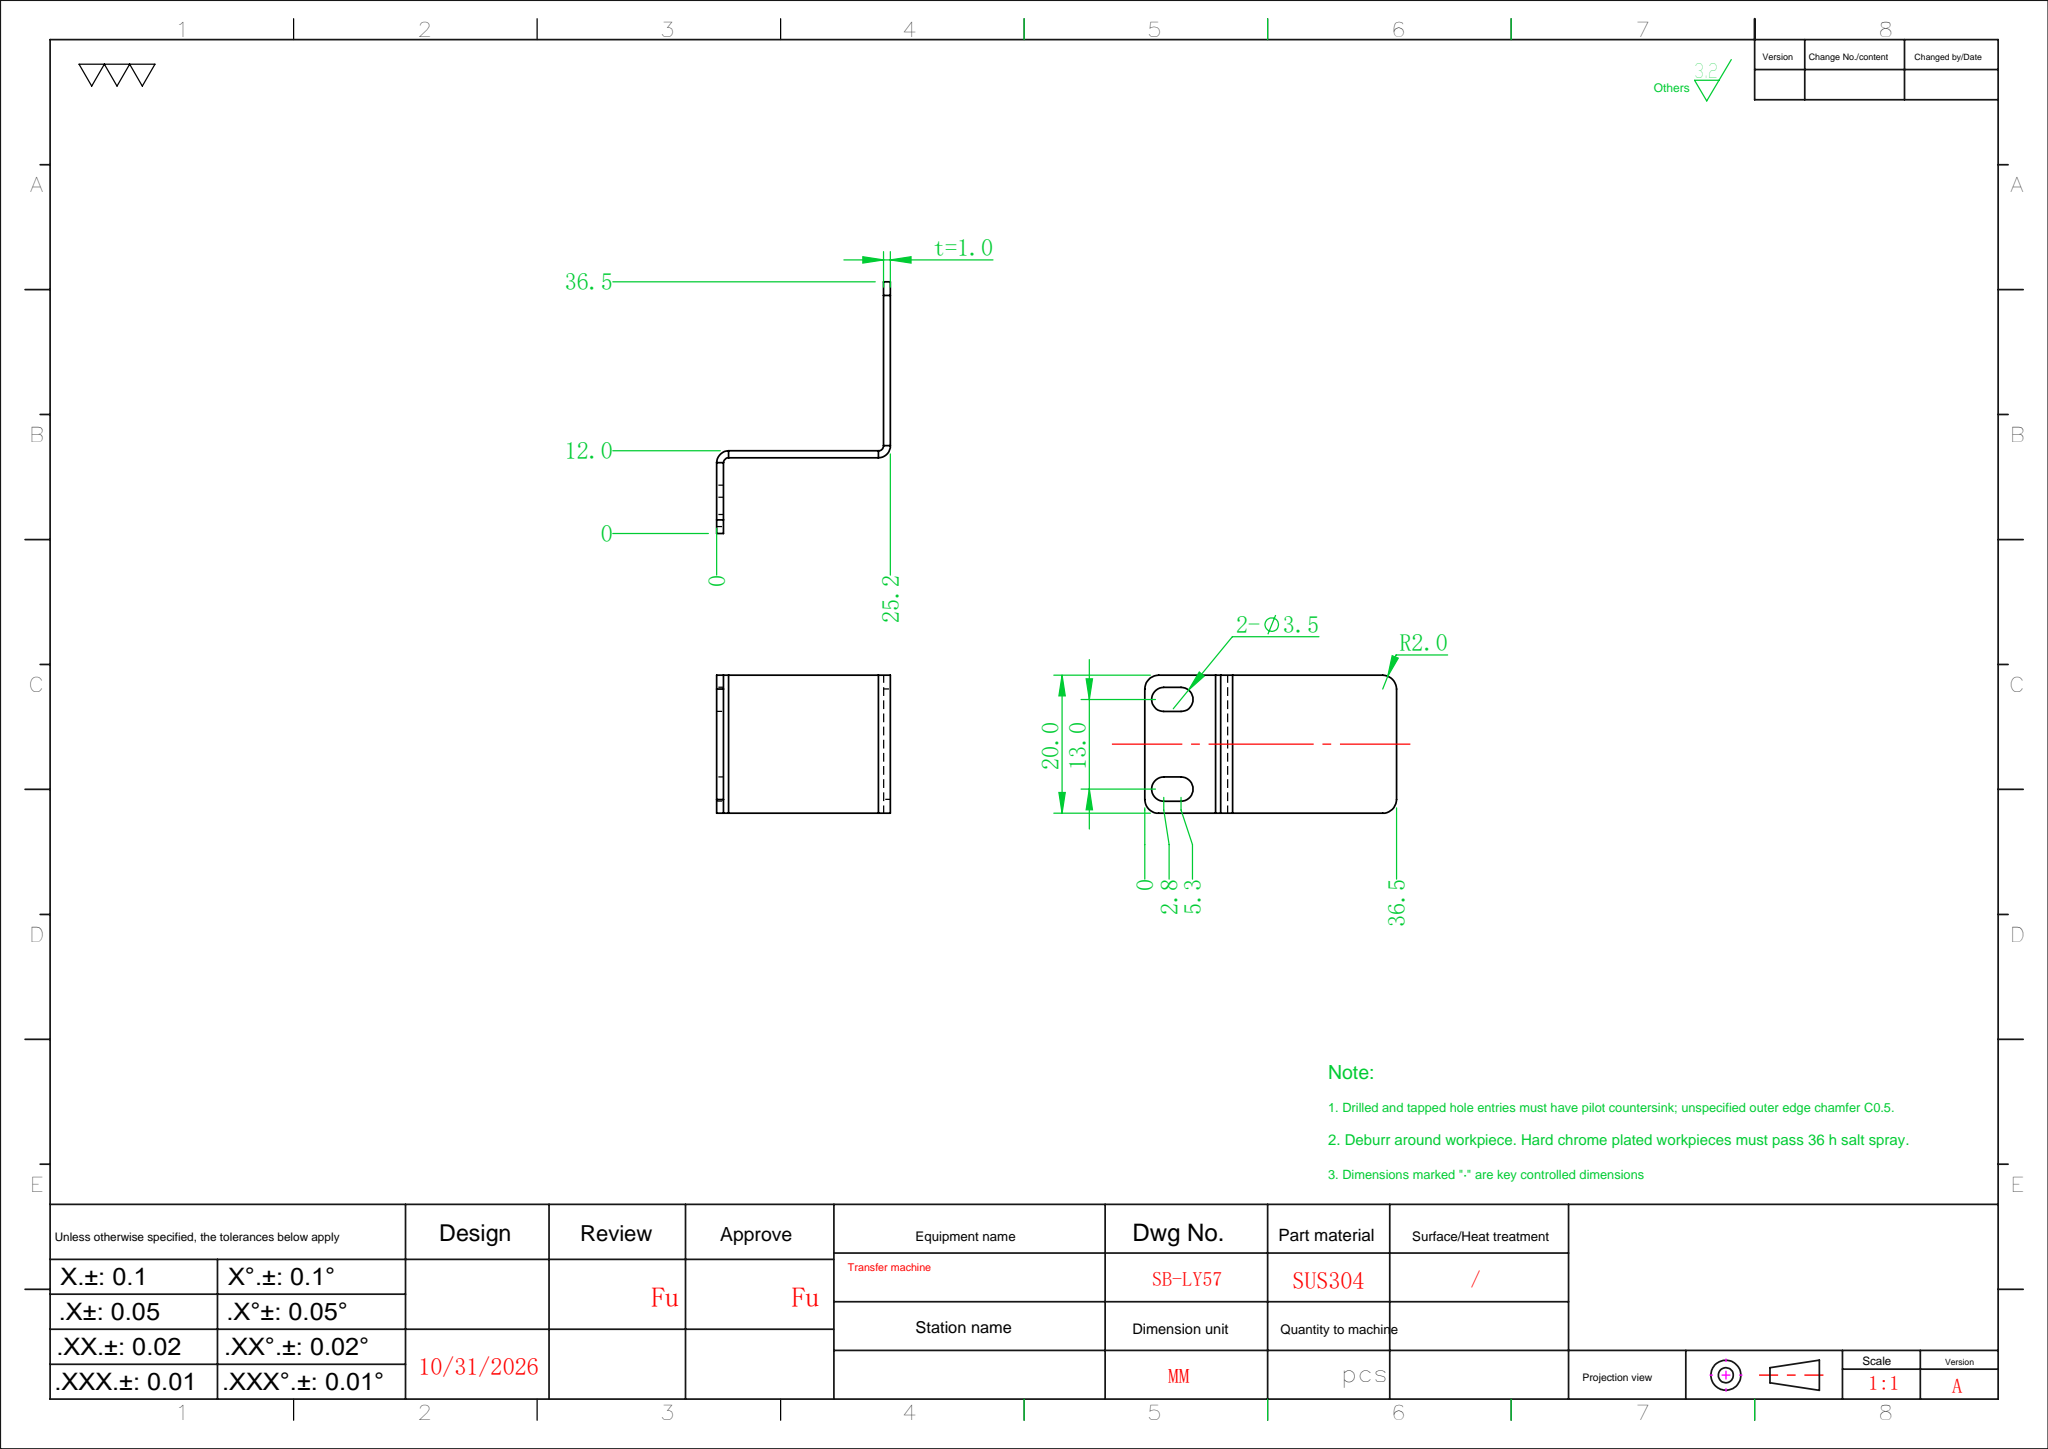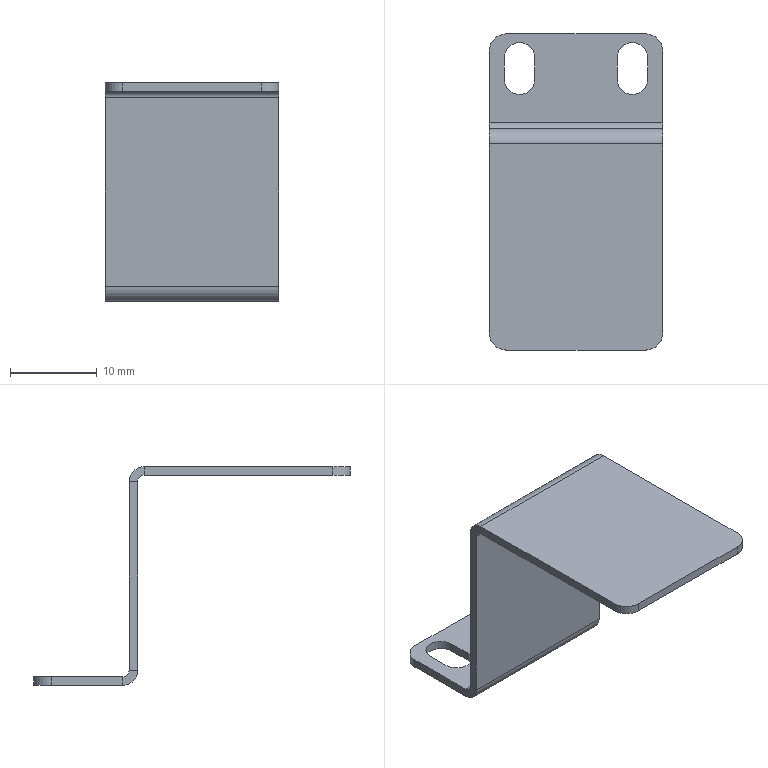Part | SolidWorks | features EdgeFlange 2, Fillet 1, FlatPattern 1, HoleWzd 1, SMBaseFlange 1, SheetMetal 1 | 1 solid | 34 faces | box 20 x 36.5 x 25.2 mm | volume 1153 mm3 | plane 22 | cylinder 12 | commonest cylinder face diameters 3.5 x4 4 x4 1.473 x2 3.473 x2
STEP:
#1=CARTESIAN_POINT('',(-10.,-6.,22.463));
#2=VERTEX_POINT('',#1);
#3=CARTESIAN_POINT('',(-10.,-5.,22.463));
#4=VERTEX_POINT('',#3);
#5=CARTESIAN_POINT('',(-10.,-6.,22.463));
#6=DIRECTION('',(0.,1.,0.));
#7=VECTOR('',#6,1000.);
#8=LINE('',#5,#7);
#9=EDGE_CURVE('',#2,#4,#8,.T.);
#10=ORIENTED_EDGE('',*,*,#9,.T.);
#11=CARTESIAN_POINT('',(-10.,-5.,0.7366));
#12=VERTEX_POINT('',#11);
#13=CARTESIAN_POINT('',(-10.,-5.,0.));
#14=DIRECTION('',(0.,0.,-1.));
#15=VECTOR('',#14,1000.);
#16=LINE('',#13,#15);
#17=EDGE_CURVE('',#4,#12,#16,.T.);
#18=ORIENTED_EDGE('',*,*,#17,.T.);
#19=CARTESIAN_POINT('',(-10.,-6.,0.7366));
#20=VERTEX_POINT('',#19);
#21=CARTESIAN_POINT('',(-10.,-6.,0.7366));
#22=DIRECTION('',(0.,-1.,0.));
#23=VECTOR('',#22,1000.);
#24=LINE('',#21,#23);
#25=EDGE_CURVE('',#12,#20,#24,.T.);
#26=ORIENTED_EDGE('',*,*,#25,.T.);
#27=CARTESIAN_POINT('',(-10.,-6.,0.));
#28=DIRECTION('',(0.,0.,-1.));
#29=VECTOR('',#28,1000.);
#30=LINE('',#27,#29);
#31=EDGE_CURVE('',#2,#20,#30,.T.);
#32=ORIENTED_EDGE('',*,*,#31,.F.);
#33=EDGE_LOOP('',(#10,#18,#26,#32));
#34=FACE_OUTER_BOUND('',#33,.T.);
#35=CARTESIAN_POINT('',(-10.,-6.,0.));
#36=DIRECTION('',(1.,0.,0.));
#37=DIRECTION('',(0.,0.,-1.));
#38=AXIS2_PLACEMENT_3D('',#35,#36,#37);
#39=PLANE('',#38);
#40=ADVANCED_FACE('',(#34),#39,.F.);
#41=CARTESIAN_POINT('',(10.,-6.,22.463));
#42=VERTEX_POINT('',#41);
#43=CARTESIAN_POINT('',(10.,-5.,22.463));
#44=VERTEX_POINT('',#43);
#45=CARTESIAN_POINT('',(10.,-6.,22.463));
#46=DIRECTION('',(0.,1.,0.));
#47=VECTOR('',#46,1000.);
#48=LINE('',#45,#47);
#49=EDGE_CURVE('',#42,#44,#48,.T.);
#50=ORIENTED_EDGE('',*,*,#49,.F.);
#51=CARTESIAN_POINT('',(10.,-6.,0.7366));
#52=VERTEX_POINT('',#51);
#53=CARTESIAN_POINT('',(10.,-6.,0.));
#54=DIRECTION('',(0.,0.,1.));
#55=VECTOR('',#54,1000.);
#56=LINE('',#53,#55);
#57=EDGE_CURVE('',#52,#42,#56,.T.);
#58=ORIENTED_EDGE('',*,*,#57,.F.);
#59=CARTESIAN_POINT('',(10.,-5.,0.7366));
#60=VERTEX_POINT('',#59);
#61=CARTESIAN_POINT('',(10.,-5.,0.7366));
#62=DIRECTION('',(0.,-1.,0.));
#63=VECTOR('',#62,1000.);
#64=LINE('',#61,#63);
#65=EDGE_CURVE('',#60,#52,#64,.T.);
#66=ORIENTED_EDGE('',*,*,#65,.F.);
#67=CARTESIAN_POINT('',(10.,-5.,24.2));
#68=DIRECTION('',(0.,0.,1.));
#69=VECTOR('',#68,1000.);
#70=LINE('',#67,#69);
#71=EDGE_CURVE('',#60,#44,#70,.T.);
#72=ORIENTED_EDGE('',*,*,#71,.T.);
#73=EDGE_LOOP('',(#50,#58,#66,#72));
#74=FACE_OUTER_BOUND('',#73,.T.);
#75=CARTESIAN_POINT('',(10.,-6.,24.2));
#76=DIRECTION('',(-1.,0.,0.));
#77=DIRECTION('',(0.,0.,1.));
#78=AXIS2_PLACEMENT_3D('',#75,#76,#77);
#79=PLANE('',#78);
#80=ADVANCED_FACE('',(#74),#79,.F.);
#81=CARTESIAN_POINT('',(-10.,-6.,22.463));
#82=DIRECTION('',(1.,0.,0.));
#83=VECTOR('',#82,1000.);
#84=LINE('',#81,#83);
#85=EDGE_CURVE('',#2,#42,#84,.T.);
#86=ORIENTED_EDGE('',*,*,#85,.F.);
#87=ORIENTED_EDGE('',*,*,#31,.T.);
#88=CARTESIAN_POINT('',(-10.,-6.,0.7366));
#89=DIRECTION('',(-1.,0.,0.));
#90=VECTOR('',#89,1000.);
#91=LINE('',#88,#90);
#92=EDGE_CURVE('',#52,#20,#91,.T.);
#93=ORIENTED_EDGE('',*,*,#92,.F.);
#94=ORIENTED_EDGE('',*,*,#57,.T.);
#95=EDGE_LOOP('',(#86,#87,#93,#94));
#96=FACE_OUTER_BOUND('',#95,.T.);
#97=CARTESIAN_POINT('',(0.,-6.,0.));
#98=DIRECTION('',(0.,1.,0.));
#99=DIRECTION('',(0.,0.,1.));
#100=AXIS2_PLACEMENT_3D('',#97,#98,#99);
#101=PLANE('',#100);
#102=ADVANCED_FACE('',(#96),#101,.F.);
#103=ORIENTED_EDGE('',*,*,#17,.F.);
#104=CARTESIAN_POINT('',(-10.,-5.,22.463));
#105=DIRECTION('',(1.,0.,0.));
#106=VECTOR('',#105,1000.);
#107=LINE('',#104,#106);
#108=EDGE_CURVE('',#4,#44,#107,.T.);
#109=ORIENTED_EDGE('',*,*,#108,.T.);
#110=ORIENTED_EDGE('',*,*,#71,.F.);
#111=CARTESIAN_POINT('',(-10.,-5.,0.7366));
#112=DIRECTION('',(1.,0.,0.));
#113=VECTOR('',#112,1000.);
#114=LINE('',#111,#113);
#115=EDGE_CURVE('',#12,#60,#114,.T.);
#116=ORIENTED_EDGE('',*,*,#115,.F.);
#117=EDGE_LOOP('',(#103,#109,#110,#116));
#118=FACE_OUTER_BOUND('',#117,.T.);
#119=CARTESIAN_POINT('',(0.,-5.,0.));
#120=DIRECTION('',(0.,1.,0.));
#121=DIRECTION('',(0.,0.,1.));
#122=AXIS2_PLACEMENT_3D('',#119,#120,#121);
#123=PLANE('',#122);
#124=ADVANCED_FACE('',(#118),#123,.T.);
#125=CARTESIAN_POINT('',(8.25,3.25,-1.));
#126=VERTEX_POINT('',#125);
#127=CARTESIAN_POINT('',(4.75,3.25,-1.));
#128=VERTEX_POINT('',#127);
#129=CARTESIAN_POINT('',(6.5,3.25,-1.));
#130=DIRECTION('',(0.,0.,1.));
#131=DIRECTION('',(1.,0.,0.));
#132=AXIS2_PLACEMENT_3D('',#129,#130,#131);
#133=CIRCLE('',#132,1.75);
#134=EDGE_CURVE('',#126,#128,#133,.T.);
#135=ORIENTED_EDGE('',*,*,#134,.T.);
#136=CARTESIAN_POINT('',(4.75,0.75,-1.));
#137=VERTEX_POINT('',#136);
#138=CARTESIAN_POINT('',(4.75,0.75,-1.));
#139=DIRECTION('',(0.,1.,0.));
#140=VECTOR('',#139,1000.);
#141=LINE('',#138,#140);
#142=EDGE_CURVE('',#137,#128,#141,.T.);
#143=ORIENTED_EDGE('',*,*,#142,.F.);
#144=CARTESIAN_POINT('',(8.25,0.75,-1.));
#145=VERTEX_POINT('',#144);
#146=CARTESIAN_POINT('',(6.5,0.75,-1.));
#147=DIRECTION('',(0.,0.,1.));
#148=DIRECTION('',(1.,0.,0.));
#149=AXIS2_PLACEMENT_3D('',#146,#147,#148);
#150=CIRCLE('',#149,1.75);
#151=EDGE_CURVE('',#137,#145,#150,.T.);
#152=ORIENTED_EDGE('',*,*,#151,.T.);
#153=CARTESIAN_POINT('',(8.25,0.75,-1.));
#154=DIRECTION('',(0.,1.,0.));
#155=VECTOR('',#154,1000.);
#156=LINE('',#153,#155);
#157=EDGE_CURVE('',#145,#126,#156,.T.);
#158=ORIENTED_EDGE('',*,*,#157,.T.);
#159=EDGE_LOOP('',(#135,#143,#152,#158));
#160=FACE_BOUND('',#159,.T.);
#161=CARTESIAN_POINT('',(-8.25,0.75,-1.));
#162=VERTEX_POINT('',#161);
#163=CARTESIAN_POINT('',(-4.75,0.75,-1.));
#164=VERTEX_POINT('',#163);
#165=CARTESIAN_POINT('',(-6.5,0.75,-1.));
#166=DIRECTION('',(0.,0.,1.));
#167=DIRECTION('',(1.,0.,0.));
#168=AXIS2_PLACEMENT_3D('',#165,#166,#167);
#169=CIRCLE('',#168,1.75);
#170=EDGE_CURVE('',#162,#164,#169,.T.);
#171=ORIENTED_EDGE('',*,*,#170,.T.);
#172=CARTESIAN_POINT('',(-4.75,3.25,-1.));
#173=VERTEX_POINT('',#172);
#174=CARTESIAN_POINT('',(-4.75,0.75,-1.));
#175=DIRECTION('',(0.,1.,0.));
#176=VECTOR('',#175,1000.);
#177=LINE('',#174,#176);
#178=EDGE_CURVE('',#164,#173,#177,.T.);
#179=ORIENTED_EDGE('',*,*,#178,.T.);
#180=CARTESIAN_POINT('',(-8.25,3.25,-1.));
#181=VERTEX_POINT('',#180);
#182=CARTESIAN_POINT('',(-6.5,3.25,-1.));
#183=DIRECTION('',(0.,0.,1.));
#184=DIRECTION('',(1.,0.,0.));
#185=AXIS2_PLACEMENT_3D('',#182,#183,#184);
#186=CIRCLE('',#185,1.75);
#187=EDGE_CURVE('',#173,#181,#186,.T.);
#188=ORIENTED_EDGE('',*,*,#187,.T.);
#189=CARTESIAN_POINT('',(-8.25,0.75,-1.));
#190=DIRECTION('',(0.,1.,0.));
#191=VECTOR('',#190,1000.);
#192=LINE('',#189,#191);
#193=EDGE_CURVE('',#162,#181,#192,.T.);
#194=ORIENTED_EDGE('',*,*,#193,.F.);
#195=EDGE_LOOP('',(#171,#179,#188,#194));
#196=FACE_BOUND('',#195,.T.);
#197=CARTESIAN_POINT('',(-10.,4.,-1.));
#198=VERTEX_POINT('',#197);
#199=CARTESIAN_POINT('',(-10.,-4.263,-1.));
#200=VERTEX_POINT('',#199);
#201=CARTESIAN_POINT('',(-10.,-6.,-1.));
#202=DIRECTION('',(0.,-1.,0.));
#203=VECTOR('',#202,1000.);
#204=LINE('',#201,#203);
#205=EDGE_CURVE('',#198,#200,#204,.T.);
#206=ORIENTED_EDGE('',*,*,#205,.F.);
#207=CARTESIAN_POINT('',(-8.,6.,-1.));
#208=VERTEX_POINT('',#207);
#209=CARTESIAN_POINT('',(-8.,4.,-1.));
#210=DIRECTION('',(0.,0.,-1.));
#211=DIRECTION('',(-1.,0.,0.));
#212=AXIS2_PLACEMENT_3D('',#209,#210,#211);
#213=CIRCLE('',#212,2.);
#214=EDGE_CURVE('',#198,#208,#213,.T.);
#215=ORIENTED_EDGE('',*,*,#214,.T.);
#216=CARTESIAN_POINT('',(8.,6.,-1.));
#217=VERTEX_POINT('',#216);
#218=CARTESIAN_POINT('',(-10.,6.,-1.));
#219=DIRECTION('',(-1.,0.,0.));
#220=VECTOR('',#219,1000.);
#221=LINE('',#218,#220);
#222=EDGE_CURVE('',#217,#208,#221,.T.);
#223=ORIENTED_EDGE('',*,*,#222,.F.);
#224=CARTESIAN_POINT('',(10.,4.,-1.));
#225=VERTEX_POINT('',#224);
#226=CARTESIAN_POINT('',(8.,4.,-1.));
#227=DIRECTION('',(0.,0.,-1.));
#228=DIRECTION('',(-1.,0.,0.));
#229=AXIS2_PLACEMENT_3D('',#226,#227,#228);
#230=CIRCLE('',#229,2.);
#231=EDGE_CURVE('',#217,#225,#230,.T.);
#232=ORIENTED_EDGE('',*,*,#231,.T.);
#233=CARTESIAN_POINT('',(10.,-4.263,-1.));
#234=VERTEX_POINT('',#233);
#235=CARTESIAN_POINT('',(10.,-6.,-1.));
#236=DIRECTION('',(0.,1.,0.));
#237=VECTOR('',#236,1000.);
#238=LINE('',#235,#237);
#239=EDGE_CURVE('',#234,#225,#238,.T.);
#240=ORIENTED_EDGE('',*,*,#239,.F.);
#241=CARTESIAN_POINT('',(10.,-4.263,-1.));
#242=DIRECTION('',(-1.,0.,0.));
#243=VECTOR('',#242,1000.);
#244=LINE('',#241,#243);
#245=EDGE_CURVE('',#234,#200,#244,.T.);
#246=ORIENTED_EDGE('',*,*,#245,.T.);
#247=EDGE_LOOP('',(#206,#215,#223,#232,#240,#246));
#248=FACE_OUTER_BOUND('',#247,.T.);
#249=CARTESIAN_POINT('',(0.,0.,-1.));
#250=DIRECTION('',(0.,0.,-1.));
#251=DIRECTION('',(-1.,0.,0.));
#252=AXIS2_PLACEMENT_3D('',#249,#250,#251);
#253=PLANE('',#252);
#254=ADVANCED_FACE('',(#160,#196,#248),#253,.T.);
#255=ORIENTED_EDGE('',*,*,#239,.T.);
#256=CARTESIAN_POINT('',(10.,4.,0.));
#257=VERTEX_POINT('',#256);
#258=CARTESIAN_POINT('',(10.,4.,-1.));
#259=DIRECTION('',(0.,0.,1.));
#260=VECTOR('',#259,1000.);
#261=LINE('',#258,#260);
#262=EDGE_CURVE('',#225,#257,#261,.T.);
#263=ORIENTED_EDGE('',*,*,#262,.T.);
#264=CARTESIAN_POINT('',(10.,-4.263,0.));
#265=VERTEX_POINT('',#264);
#266=CARTESIAN_POINT('',(10.,-6.,0.));
#267=DIRECTION('',(0.,1.,0.));
#268=VECTOR('',#267,1000.);
#269=LINE('',#266,#268);
#270=EDGE_CURVE('',#265,#257,#269,.T.);
#271=ORIENTED_EDGE('',*,*,#270,.F.);
#272=CARTESIAN_POINT('',(10.,-4.263,0.));
#273=DIRECTION('',(0.,0.,-1.));
#274=VECTOR('',#273,1000.);
#275=LINE('',#272,#274);
#276=EDGE_CURVE('',#265,#234,#275,.T.);
#277=ORIENTED_EDGE('',*,*,#276,.T.);
#278=EDGE_LOOP('',(#255,#263,#271,#277));
#279=FACE_OUTER_BOUND('',#278,.T.);
#280=CARTESIAN_POINT('',(10.,-6.,-1.));
#281=DIRECTION('',(1.,0.,0.));
#282=DIRECTION('',(0.,0.,-1.));
#283=AXIS2_PLACEMENT_3D('',#280,#281,#282);
#284=PLANE('',#283);
#285=ADVANCED_FACE('',(#279),#284,.T.);
#286=CARTESIAN_POINT('',(8.25,3.25,0.));
#287=VERTEX_POINT('',#286);
#288=CARTESIAN_POINT('',(4.75,3.25,0.));
#289=VERTEX_POINT('',#288);
#290=CARTESIAN_POINT('',(6.5,3.25,0.));
#291=DIRECTION('',(0.,0.,1.));
#292=DIRECTION('',(1.,0.,0.));
#293=AXIS2_PLACEMENT_3D('',#290,#291,#292);
#294=CIRCLE('',#293,1.75);
#295=EDGE_CURVE('',#287,#289,#294,.T.);
#296=ORIENTED_EDGE('',*,*,#295,.F.);
#297=CARTESIAN_POINT('',(8.25,0.75,0.));
#298=VERTEX_POINT('',#297);
#299=CARTESIAN_POINT('',(8.25,0.75,0.));
#300=DIRECTION('',(0.,1.,0.));
#301=VECTOR('',#300,1000.);
#302=LINE('',#299,#301);
#303=EDGE_CURVE('',#298,#287,#302,.T.);
#304=ORIENTED_EDGE('',*,*,#303,.F.);
#305=CARTESIAN_POINT('',(4.75,0.75,0.));
#306=VERTEX_POINT('',#305);
#307=CARTESIAN_POINT('',(6.5,0.75,0.));
#308=DIRECTION('',(0.,0.,1.));
#309=DIRECTION('',(1.,0.,0.));
#310=AXIS2_PLACEMENT_3D('',#307,#308,#309);
#311=CIRCLE('',#310,1.75);
#312=EDGE_CURVE('',#306,#298,#311,.T.);
#313=ORIENTED_EDGE('',*,*,#312,.F.);
#314=CARTESIAN_POINT('',(4.75,0.75,0.));
#315=DIRECTION('',(0.,1.,0.));
#316=VECTOR('',#315,1000.);
#317=LINE('',#314,#316);
#318=EDGE_CURVE('',#306,#289,#317,.T.);
#319=ORIENTED_EDGE('',*,*,#318,.T.);
#320=EDGE_LOOP('',(#296,#304,#313,#319));
#321=FACE_BOUND('',#320,.T.);
#322=CARTESIAN_POINT('',(-8.25,0.75,0.));
#323=VERTEX_POINT('',#322);
#324=CARTESIAN_POINT('',(-8.25,3.25,0.));
#325=VERTEX_POINT('',#324);
#326=CARTESIAN_POINT('',(-8.25,0.75,0.));
#327=DIRECTION('',(0.,1.,0.));
#328=VECTOR('',#327,1000.);
#329=LINE('',#326,#328);
#330=EDGE_CURVE('',#323,#325,#329,.T.);
#331=ORIENTED_EDGE('',*,*,#330,.T.);
#332=CARTESIAN_POINT('',(-4.75,3.25,0.));
#333=VERTEX_POINT('',#332);
#334=CARTESIAN_POINT('',(-6.5,3.25,0.));
#335=DIRECTION('',(0.,0.,1.));
#336=DIRECTION('',(1.,0.,0.));
#337=AXIS2_PLACEMENT_3D('',#334,#335,#336);
#338=CIRCLE('',#337,1.75);
#339=EDGE_CURVE('',#333,#325,#338,.T.);
#340=ORIENTED_EDGE('',*,*,#339,.F.);
#341=CARTESIAN_POINT('',(-4.75,0.75,0.));
#342=VERTEX_POINT('',#341);
#343=CARTESIAN_POINT('',(-4.75,0.75,0.));
#344=DIRECTION('',(0.,1.,0.));
#345=VECTOR('',#344,1000.);
#346=LINE('',#343,#345);
#347=EDGE_CURVE('',#342,#333,#346,.T.);
#348=ORIENTED_EDGE('',*,*,#347,.F.);
#349=CARTESIAN_POINT('',(-6.5,0.75,0.));
#350=DIRECTION('',(0.,0.,1.));
#351=DIRECTION('',(1.,0.,0.));
#352=AXIS2_PLACEMENT_3D('',#349,#350,#351);
#353=CIRCLE('',#352,1.75);
#354=EDGE_CURVE('',#323,#342,#353,.T.);
#355=ORIENTED_EDGE('',*,*,#354,.F.);
#356=EDGE_LOOP('',(#331,#340,#348,#355));
#357=FACE_BOUND('',#356,.T.);
#358=CARTESIAN_POINT('',(8.,6.,0.));
#359=VERTEX_POINT('',#358);
#360=CARTESIAN_POINT('',(-8.,6.,0.));
#361=VERTEX_POINT('',#360);
#362=CARTESIAN_POINT('',(-10.,6.,0.));
#363=DIRECTION('',(-1.,0.,0.));
#364=VECTOR('',#363,1000.);
#365=LINE('',#362,#364);
#366=EDGE_CURVE('',#359,#361,#365,.T.);
#367=ORIENTED_EDGE('',*,*,#366,.T.);
#368=CARTESIAN_POINT('',(-10.,4.,0.));
#369=VERTEX_POINT('',#368);
#370=CARTESIAN_POINT('',(-8.,4.,0.));
#371=DIRECTION('',(0.,0.,1.));
#372=DIRECTION('',(-1.,0.,0.));
#373=AXIS2_PLACEMENT_3D('',#370,#371,#372);
#374=CIRCLE('',#373,2.);
#375=EDGE_CURVE('',#361,#369,#374,.T.);
#376=ORIENTED_EDGE('',*,*,#375,.T.);
#377=CARTESIAN_POINT('',(-10.,-4.263,0.));
#378=VERTEX_POINT('',#377);
#379=CARTESIAN_POINT('',(-10.,-6.,0.));
#380=DIRECTION('',(0.,-1.,0.));
#381=VECTOR('',#380,1000.);
#382=LINE('',#379,#381);
#383=EDGE_CURVE('',#369,#378,#382,.T.);
#384=ORIENTED_EDGE('',*,*,#383,.T.);
#385=CARTESIAN_POINT('',(10.,-4.263,0.));
#386=DIRECTION('',(-1.,0.,0.));
#387=VECTOR('',#386,1000.);
#388=LINE('',#385,#387);
#389=EDGE_CURVE('',#265,#378,#388,.T.);
#390=ORIENTED_EDGE('',*,*,#389,.F.);
#391=ORIENTED_EDGE('',*,*,#270,.T.);
#392=CARTESIAN_POINT('',(8.,4.,0.));
#393=DIRECTION('',(0.,0.,1.));
#394=DIRECTION('',(-1.,0.,0.));
#395=AXIS2_PLACEMENT_3D('',#392,#393,#394);
#396=CIRCLE('',#395,2.);
#397=EDGE_CURVE('',#257,#359,#396,.T.);
#398=ORIENTED_EDGE('',*,*,#397,.T.);
#399=EDGE_LOOP('',(#367,#376,#384,#390,#391,#398));
#400=FACE_OUTER_BOUND('',#399,.T.);
#401=CARTESIAN_POINT('',(0.,0.,0.));
#402=DIRECTION('',(0.,0.,-1.));
#403=DIRECTION('',(-1.,0.,0.));
#404=AXIS2_PLACEMENT_3D('',#401,#402,#403);
#405=PLANE('',#404);
#406=ADVANCED_FACE('',(#321,#357,#400),#405,.F.);
#407=ORIENTED_EDGE('',*,*,#383,.F.);
#408=CARTESIAN_POINT('',(-10.,4.,-1.));
#409=DIRECTION('',(0.,0.,-1.));
#410=VECTOR('',#409,1000.);
#411=LINE('',#408,#410);
#412=EDGE_CURVE('',#369,#198,#411,.T.);
#413=ORIENTED_EDGE('',*,*,#412,.T.);
#414=ORIENTED_EDGE('',*,*,#205,.T.);
#415=CARTESIAN_POINT('',(-10.,-4.263,0.));
#416=DIRECTION('',(0.,0.,-1.));
#417=VECTOR('',#416,1000.);
#418=LINE('',#415,#417);
#419=EDGE_CURVE('',#378,#200,#418,.T.);
#420=ORIENTED_EDGE('',*,*,#419,.F.);
#421=EDGE_LOOP('',(#407,#413,#414,#420));
#422=FACE_OUTER_BOUND('',#421,.T.);
#423=CARTESIAN_POINT('',(-10.,-6.,-1.));
#424=DIRECTION('',(-1.,0.,0.));
#425=DIRECTION('',(0.,0.,1.));
#426=AXIS2_PLACEMENT_3D('',#423,#424,#425);
#427=PLANE('',#426);
#428=ADVANCED_FACE('',(#422),#427,.T.);
#429=ORIENTED_EDGE('',*,*,#222,.T.);
#430=CARTESIAN_POINT('',(-8.,6.,-1.));
#431=DIRECTION('',(0.,0.,1.));
#432=VECTOR('',#431,1000.);
#433=LINE('',#430,#432);
#434=EDGE_CURVE('',#208,#361,#433,.T.);
#435=ORIENTED_EDGE('',*,*,#434,.T.);
#436=ORIENTED_EDGE('',*,*,#366,.F.);
#437=CARTESIAN_POINT('',(8.,6.,-1.));
#438=DIRECTION('',(0.,0.,-1.));
#439=VECTOR('',#438,1000.);
#440=LINE('',#437,#439);
#441=EDGE_CURVE('',#359,#217,#440,.T.);
#442=ORIENTED_EDGE('',*,*,#441,.T.);
#443=EDGE_LOOP('',(#429,#435,#436,#442));
#444=FACE_OUTER_BOUND('',#443,.T.);
#445=CARTESIAN_POINT('',(-10.,6.,-1.));
#446=DIRECTION('',(0.,1.,0.));
#447=DIRECTION('',(0.,0.,1.));
#448=AXIS2_PLACEMENT_3D('',#445,#446,#447);
#449=PLANE('',#448);
#450=ADVANCED_FACE('',(#444),#449,.T.);
#451=ORIENTED_EDGE('',*,*,#134,.F.);
#452=CARTESIAN_POINT('',(8.25,3.25,-1.));
#453=DIRECTION('',(0.,0.,-1.));
#454=VECTOR('',#453,1000.);
#455=LINE('',#452,#454);
#456=EDGE_CURVE('',#287,#126,#455,.T.);
#457=ORIENTED_EDGE('',*,*,#456,.F.);
#458=ORIENTED_EDGE('',*,*,#295,.T.);
#459=CARTESIAN_POINT('',(4.75,3.25,0.));
#460=DIRECTION('',(0.,0.,1.));
#461=VECTOR('',#460,1000.);
#462=LINE('',#459,#461);
#463=EDGE_CURVE('',#128,#289,#462,.T.);
#464=ORIENTED_EDGE('',*,*,#463,.F.);
#465=EDGE_LOOP('',(#451,#457,#458,#464));
#466=FACE_OUTER_BOUND('',#465,.T.);
#467=CARTESIAN_POINT('',(6.5,3.25,0.));
#468=DIRECTION('',(0.,0.,1.));
#469=DIRECTION('',(1.,0.,0.));
#470=AXIS2_PLACEMENT_3D('',#467,#468,#469);
#471=CYLINDRICAL_SURFACE('',#470,1.75);
#472=ADVANCED_FACE('',(#466),#471,.F.);
#473=ORIENTED_EDGE('',*,*,#312,.T.);
#474=CARTESIAN_POINT('',(8.25,0.75,-1.));
#475=DIRECTION('',(0.,0.,-1.));
#476=VECTOR('',#475,1000.);
#477=LINE('',#474,#476);
#478=EDGE_CURVE('',#298,#145,#477,.T.);
#479=ORIENTED_EDGE('',*,*,#478,.T.);
#480=ORIENTED_EDGE('',*,*,#151,.F.);
#481=CARTESIAN_POINT('',(4.75,0.75,0.));
#482=DIRECTION('',(0.,0.,-1.));
#483=VECTOR('',#482,1000.);
#484=LINE('',#481,#483);
#485=EDGE_CURVE('',#306,#137,#484,.T.);
#486=ORIENTED_EDGE('',*,*,#485,.F.);
#487=EDGE_LOOP('',(#473,#479,#480,#486));
#488=FACE_OUTER_BOUND('',#487,.T.);
#489=CARTESIAN_POINT('',(6.5,0.75,0.));
#490=DIRECTION('',(0.,0.,1.));
#491=DIRECTION('',(1.,0.,0.));
#492=AXIS2_PLACEMENT_3D('',#489,#490,#491);
#493=CYLINDRICAL_SURFACE('',#492,1.75);
#494=ADVANCED_FACE('',(#488),#493,.F.);
#495=ORIENTED_EDGE('',*,*,#463,.T.);
#496=ORIENTED_EDGE('',*,*,#318,.F.);
#497=ORIENTED_EDGE('',*,*,#485,.T.);
#498=ORIENTED_EDGE('',*,*,#142,.T.);
#499=EDGE_LOOP('',(#495,#496,#497,#498));
#500=FACE_OUTER_BOUND('',#499,.T.);
#501=CARTESIAN_POINT('',(4.75,0.75,0.));
#502=DIRECTION('',(-1.,0.,0.));
#503=DIRECTION('',(0.,0.,1.));
#504=AXIS2_PLACEMENT_3D('',#501,#502,#503);
#505=PLANE('',#504);
#506=ADVANCED_FACE('',(#500),#505,.F.);
#507=ORIENTED_EDGE('',*,*,#456,.T.);
#508=ORIENTED_EDGE('',*,*,#157,.F.);
#509=ORIENTED_EDGE('',*,*,#478,.F.);
#510=ORIENTED_EDGE('',*,*,#303,.T.);
#511=EDGE_LOOP('',(#507,#508,#509,#510));
#512=FACE_OUTER_BOUND('',#511,.T.);
#513=CARTESIAN_POINT('',(8.25,0.75,-1.));
#514=DIRECTION('',(1.,0.,0.));
#515=DIRECTION('',(0.,0.,-1.));
#516=AXIS2_PLACEMENT_3D('',#513,#514,#515);
#517=PLANE('',#516);
#518=ADVANCED_FACE('',(#512),#517,.F.);
#519=ORIENTED_EDGE('',*,*,#187,.F.);
#520=CARTESIAN_POINT('',(-4.75,3.25,-1.));
#521=DIRECTION('',(0.,0.,-1.));
#522=VECTOR('',#521,1000.);
#523=LINE('',#520,#522);
#524=EDGE_CURVE('',#333,#173,#523,.T.);
#525=ORIENTED_EDGE('',*,*,#524,.F.);
#526=ORIENTED_EDGE('',*,*,#339,.T.);
#527=CARTESIAN_POINT('',(-8.25,3.25,0.));
#528=DIRECTION('',(0.,0.,1.));
#529=VECTOR('',#528,1000.);
#530=LINE('',#527,#529);
#531=EDGE_CURVE('',#181,#325,#530,.T.);
#532=ORIENTED_EDGE('',*,*,#531,.F.);
#533=EDGE_LOOP('',(#519,#525,#526,#532));
#534=FACE_OUTER_BOUND('',#533,.T.);
#535=CARTESIAN_POINT('',(-6.5,3.25,0.));
#536=DIRECTION('',(0.,0.,1.));
#537=DIRECTION('',(1.,0.,0.));
#538=AXIS2_PLACEMENT_3D('',#535,#536,#537);
#539=CYLINDRICAL_SURFACE('',#538,1.75);
#540=ADVANCED_FACE('',(#534),#539,.F.);
#541=ORIENTED_EDGE('',*,*,#354,.T.);
#542=CARTESIAN_POINT('',(-4.75,0.75,-1.));
#543=DIRECTION('',(0.,0.,-1.));
#544=VECTOR('',#543,1000.);
#545=LINE('',#542,#544);
#546=EDGE_CURVE('',#342,#164,#545,.T.);
#547=ORIENTED_EDGE('',*,*,#546,.T.);
#548=ORIENTED_EDGE('',*,*,#170,.F.);
#549=CARTESIAN_POINT('',(-8.25,0.75,0.));
#550=DIRECTION('',(0.,0.,-1.));
#551=VECTOR('',#550,1000.);
#552=LINE('',#549,#551);
#553=EDGE_CURVE('',#323,#162,#552,.T.);
#554=ORIENTED_EDGE('',*,*,#553,.F.);
#555=EDGE_LOOP('',(#541,#547,#548,#554));
#556=FACE_OUTER_BOUND('',#555,.T.);
#557=CARTESIAN_POINT('',(-6.5,0.75,0.));
#558=DIRECTION('',(0.,0.,1.));
#559=DIRECTION('',(1.,0.,0.));
#560=AXIS2_PLACEMENT_3D('',#557,#558,#559);
#561=CYLINDRICAL_SURFACE('',#560,1.75);
#562=ADVANCED_FACE('',(#556),#561,.F.);
#563=ORIENTED_EDGE('',*,*,#531,.T.);
#564=ORIENTED_EDGE('',*,*,#330,.F.);
#565=ORIENTED_EDGE('',*,*,#553,.T.);
#566=ORIENTED_EDGE('',*,*,#193,.T.);
#567=EDGE_LOOP('',(#563,#564,#565,#566));
#568=FACE_OUTER_BOUND('',#567,.T.);
#569=CARTESIAN_POINT('',(-8.25,0.75,0.));
#570=DIRECTION('',(-1.,0.,0.));
#571=DIRECTION('',(0.,0.,1.));
#572=AXIS2_PLACEMENT_3D('',#569,#570,#571);
#573=PLANE('',#572);
#574=ADVANCED_FACE('',(#568),#573,.F.);
#575=ORIENTED_EDGE('',*,*,#524,.T.);
#576=ORIENTED_EDGE('',*,*,#178,.F.);
#577=ORIENTED_EDGE('',*,*,#546,.F.);
#578=ORIENTED_EDGE('',*,*,#347,.T.);
#579=EDGE_LOOP('',(#575,#576,#577,#578));
#580=FACE_OUTER_BOUND('',#579,.T.);
#581=CARTESIAN_POINT('',(-4.75,0.75,-1.));
#582=DIRECTION('',(1.,0.,0.));
#583=DIRECTION('',(0.,0.,-1.));
#584=AXIS2_PLACEMENT_3D('',#581,#582,#583);
#585=PLANE('',#584);
#586=ADVANCED_FACE('',(#580),#585,.F.);
#587=ORIENTED_EDGE('',*,*,#25,.F.);
#588=CARTESIAN_POINT('',(-10.,-4.263,0.7366));
#589=DIRECTION('',(-1.,0.,0.));
#590=DIRECTION('',(0.,0.,-1.));
#591=AXIS2_PLACEMENT_3D('',#588,#589,#590);
#592=CIRCLE('',#591,0.7366);
#593=EDGE_CURVE('',#378,#12,#592,.T.);
#594=ORIENTED_EDGE('',*,*,#593,.F.);
#595=ORIENTED_EDGE('',*,*,#419,.T.);
#596=CARTESIAN_POINT('',(-10.,-4.263,0.7366));
#597=DIRECTION('',(-1.,0.,0.));
#598=DIRECTION('',(0.,0.,-1.));
#599=AXIS2_PLACEMENT_3D('',#596,#597,#598);
#600=CIRCLE('',#599,1.737);
#601=EDGE_CURVE('',#200,#20,#600,.T.);
#602=ORIENTED_EDGE('',*,*,#601,.T.);
#603=EDGE_LOOP('',(#587,#594,#595,#602));
#604=FACE_OUTER_BOUND('',#603,.T.);
#605=CARTESIAN_POINT('',(-10.,-4.263,0.7366));
#606=DIRECTION('',(-1.,0.,0.));
#607=DIRECTION('',(0.,0.,1.));
#608=AXIS2_PLACEMENT_3D('',#605,#606,#607);
#609=PLANE('',#608);
#610=ADVANCED_FACE('',(#604),#609,.T.);
#611=CARTESIAN_POINT('',(10.,-4.263,0.7366));
#612=DIRECTION('',(1.,0.,0.));
#613=DIRECTION('',(0.,0.,-1.));
#614=AXIS2_PLACEMENT_3D('',#611,#612,#613);
#615=CIRCLE('',#614,0.7366);
#616=EDGE_CURVE('',#60,#265,#615,.T.);
#617=ORIENTED_EDGE('',*,*,#616,.F.);
#618=ORIENTED_EDGE('',*,*,#65,.T.);
#619=CARTESIAN_POINT('',(10.,-4.263,0.7366));
#620=DIRECTION('',(1.,0.,0.));
#621=DIRECTION('',(0.,0.,-1.));
#622=AXIS2_PLACEMENT_3D('',#619,#620,#621);
#623=CIRCLE('',#622,1.737);
#624=EDGE_CURVE('',#52,#234,#623,.T.);
#625=ORIENTED_EDGE('',*,*,#624,.T.);
#626=ORIENTED_EDGE('',*,*,#276,.F.);
#627=EDGE_LOOP('',(#617,#618,#625,#626));
#628=FACE_OUTER_BOUND('',#627,.T.);
#629=CARTESIAN_POINT('',(10.,-4.263,0.7366));
#630=DIRECTION('',(-1.,0.,0.));
#631=DIRECTION('',(0.,0.,1.));
#632=AXIS2_PLACEMENT_3D('',#629,#630,#631);
#633=PLANE('',#632);
#634=ADVANCED_FACE('',(#628),#633,.F.);
#635=ORIENTED_EDGE('',*,*,#245,.F.);
#636=ORIENTED_EDGE('',*,*,#624,.F.);
#637=ORIENTED_EDGE('',*,*,#92,.T.);
#638=ORIENTED_EDGE('',*,*,#601,.F.);
#639=EDGE_LOOP('',(#635,#636,#637,#638));
#640=FACE_OUTER_BOUND('',#639,.T.);
#641=CARTESIAN_POINT('',(10.,-4.263,0.7366));
#642=DIRECTION('',(1.,0.,0.));
#643=DIRECTION('',(0.,-1.,0.));
#644=AXIS2_PLACEMENT_3D('',#641,#642,#643);
#645=CYLINDRICAL_SURFACE('',#644,1.737);
#646=ADVANCED_FACE('',(#640),#645,.T.);
#647=ORIENTED_EDGE('',*,*,#389,.T.);
#648=ORIENTED_EDGE('',*,*,#593,.T.);
#649=ORIENTED_EDGE('',*,*,#115,.T.);
#650=ORIENTED_EDGE('',*,*,#616,.T.);
#651=EDGE_LOOP('',(#647,#648,#649,#650));
#652=FACE_OUTER_BOUND('',#651,.T.);
#653=CARTESIAN_POINT('',(10.,-4.263,0.7366));
#654=DIRECTION('',(1.,0.,0.));
#655=DIRECTION('',(0.,-1.,0.));
#656=AXIS2_PLACEMENT_3D('',#653,#654,#655);
#657=CYLINDRICAL_SURFACE('',#656,0.7366);
#658=ADVANCED_FACE('',(#652),#657,.F.);
#659=CARTESIAN_POINT('',(10.,-6.737,23.2));
#660=VERTEX_POINT('',#659);
#661=CARTESIAN_POINT('',(10.,-6.737,24.2));
#662=VERTEX_POINT('',#661);
#663=CARTESIAN_POINT('',(10.,-6.737,24.2));
#664=DIRECTION('',(0.,0.,1.));
#665=VECTOR('',#664,1000.);
#666=LINE('',#663,#665);
#667=EDGE_CURVE('',#660,#662,#666,.T.);
#668=ORIENTED_EDGE('',*,*,#667,.F.);
#669=CARTESIAN_POINT('',(10.,-6.737,22.463));
#670=DIRECTION('',(1.,0.,0.));
#671=DIRECTION('',(0.,0.,1.));
#672=AXIS2_PLACEMENT_3D('',#669,#670,#671);
#673=CIRCLE('',#672,0.7366);
#674=EDGE_CURVE('',#42,#660,#673,.T.);
#675=ORIENTED_EDGE('',*,*,#674,.F.);
#676=ORIENTED_EDGE('',*,*,#49,.T.);
#677=CARTESIAN_POINT('',(10.,-6.737,22.463));
#678=DIRECTION('',(1.,0.,0.));
#679=DIRECTION('',(0.,0.,1.));
#680=AXIS2_PLACEMENT_3D('',#677,#678,#679);
#681=CIRCLE('',#680,1.737);
#682=EDGE_CURVE('',#44,#662,#681,.T.);
#683=ORIENTED_EDGE('',*,*,#682,.T.);
#684=EDGE_LOOP('',(#668,#675,#676,#683));
#685=FACE_OUTER_BOUND('',#684,.T.);
#686=CARTESIAN_POINT('',(10.,-6.737,22.463));
#687=DIRECTION('',(1.,0.,0.));
#688=DIRECTION('',(0.,0.,-1.));
#689=AXIS2_PLACEMENT_3D('',#686,#687,#688);
#690=PLANE('',#689);
#691=ADVANCED_FACE('',(#685),#690,.T.);
#692=CARTESIAN_POINT('',(-10.,-6.737,23.2));
#693=VERTEX_POINT('',#692);
#694=CARTESIAN_POINT('',(-10.,-6.737,22.463));
#695=DIRECTION('',(-1.,0.,0.));
#696=DIRECTION('',(0.,0.,1.));
#697=AXIS2_PLACEMENT_3D('',#694,#695,#696);
#698=CIRCLE('',#697,0.7366);
#699=EDGE_CURVE('',#693,#2,#698,.T.);
#700=ORIENTED_EDGE('',*,*,#699,.F.);
#701=CARTESIAN_POINT('',(-10.,-6.737,24.2));
#702=VERTEX_POINT('',#701);
#703=CARTESIAN_POINT('',(-10.,-6.737,23.2));
#704=DIRECTION('',(0.,0.,1.));
#705=VECTOR('',#704,1000.);
#706=LINE('',#703,#705);
#707=EDGE_CURVE('',#693,#702,#706,.T.);
#708=ORIENTED_EDGE('',*,*,#707,.T.);
#709=CARTESIAN_POINT('',(-10.,-6.737,22.463));
#710=DIRECTION('',(-1.,0.,0.));
#711=DIRECTION('',(0.,0.,1.));
#712=AXIS2_PLACEMENT_3D('',#709,#710,#711);
#713=CIRCLE('',#712,1.737);
#714=EDGE_CURVE('',#702,#4,#713,.T.);
#715=ORIENTED_EDGE('',*,*,#714,.T.);
#716=ORIENTED_EDGE('',*,*,#9,.F.);
#717=EDGE_LOOP('',(#700,#708,#715,#716));
#718=FACE_OUTER_BOUND('',#717,.T.);
#719=CARTESIAN_POINT('',(-10.,-6.737,22.463));
#720=DIRECTION('',(1.,0.,0.));
#721=DIRECTION('',(0.,0.,-1.));
#722=AXIS2_PLACEMENT_3D('',#719,#720,#721);
#723=PLANE('',#722);
#724=ADVANCED_FACE('',(#718),#723,.F.);
#725=ORIENTED_EDGE('',*,*,#108,.F.);
#726=ORIENTED_EDGE('',*,*,#714,.F.);
#727=CARTESIAN_POINT('',(0.,-6.737,24.2));
#728=DIRECTION('',(-1.,0.,0.));
#729=VECTOR('',#728,1000.);
#730=LINE('',#727,#729);
#731=EDGE_CURVE('',#662,#702,#730,.T.);
#732=ORIENTED_EDGE('',*,*,#731,.F.);
#733=ORIENTED_EDGE('',*,*,#682,.F.);
#734=EDGE_LOOP('',(#725,#726,#732,#733));
#735=FACE_OUTER_BOUND('',#734,.T.);
#736=CARTESIAN_POINT('',(-10.,-6.737,22.463));
#737=DIRECTION('',(-1.,0.,0.));
#738=DIRECTION('',(0.,0.,1.));
#739=AXIS2_PLACEMENT_3D('',#736,#737,#738);
#740=CYLINDRICAL_SURFACE('',#739,1.737);
#741=ADVANCED_FACE('',(#735),#740,.T.);
#742=ORIENTED_EDGE('',*,*,#85,.T.);
#743=ORIENTED_EDGE('',*,*,#674,.T.);
#744=CARTESIAN_POINT('',(10.,-6.737,23.2));
#745=DIRECTION('',(-1.,0.,0.));
#746=VECTOR('',#745,1000.);
#747=LINE('',#744,#746);
#748=EDGE_CURVE('',#660,#693,#747,.T.);
#749=ORIENTED_EDGE('',*,*,#748,.T.);
#750=ORIENTED_EDGE('',*,*,#699,.T.);
#751=EDGE_LOOP('',(#742,#743,#749,#750));
#752=FACE_OUTER_BOUND('',#751,.T.);
#753=CARTESIAN_POINT('',(-10.,-6.737,22.463));
#754=DIRECTION('',(-1.,0.,0.));
#755=DIRECTION('',(0.,0.,1.));
#756=AXIS2_PLACEMENT_3D('',#753,#754,#755);
#757=CYLINDRICAL_SURFACE('',#756,0.7366);
#758=ADVANCED_FACE('',(#752),#757,.F.);
#759=CARTESIAN_POINT('',(-10.,-28.5,23.2));
#760=VERTEX_POINT('',#759);
#761=CARTESIAN_POINT('',(-10.,0.,23.2));
#762=DIRECTION('',(0.,1.,0.));
#763=VECTOR('',#762,1000.);
#764=LINE('',#761,#763);
#765=EDGE_CURVE('',#760,#693,#764,.T.);
#766=ORIENTED_EDGE('',*,*,#765,.F.);
#767=CARTESIAN_POINT('',(-10.,-28.5,24.2));
#768=VERTEX_POINT('',#767);
#769=CARTESIAN_POINT('',(-10.,-28.5,24.2));
#770=DIRECTION('',(0.,0.,1.));
#771=VECTOR('',#770,1000.);
#772=LINE('',#769,#771);
#773=EDGE_CURVE('',#760,#768,#772,.T.);
#774=ORIENTED_EDGE('',*,*,#773,.T.);
#775=CARTESIAN_POINT('',(-10.,-6.,24.2));
#776=DIRECTION('',(0.,1.,0.));
#777=VECTOR('',#776,1000.);
#778=LINE('',#775,#777);
#779=EDGE_CURVE('',#768,#702,#778,.T.);
#780=ORIENTED_EDGE('',*,*,#779,.T.);
#781=ORIENTED_EDGE('',*,*,#707,.F.);
#782=EDGE_LOOP('',(#766,#774,#780,#781));
#783=FACE_OUTER_BOUND('',#782,.T.);
#784=CARTESIAN_POINT('',(-10.,-6.,24.2));
#785=DIRECTION('',(-1.,0.,0.));
#786=DIRECTION('',(0.,0.,1.));
#787=AXIS2_PLACEMENT_3D('',#784,#785,#786);
#788=PLANE('',#787);
#789=ADVANCED_FACE('',(#783),#788,.T.);
#790=CARTESIAN_POINT('',(10.,-28.5,24.2));
#791=VERTEX_POINT('',#790);
#792=CARTESIAN_POINT('',(10.,-30.5,24.2));
#793=DIRECTION('',(0.,-1.,0.));
#794=VECTOR('',#793,1000.);
#795=LINE('',#792,#794);
#796=EDGE_CURVE('',#662,#791,#795,.T.);
#797=ORIENTED_EDGE('',*,*,#796,.T.);
#798=CARTESIAN_POINT('',(10.,-28.5,23.2));
#799=VERTEX_POINT('',#798);
#800=CARTESIAN_POINT('',(10.,-28.5,24.2));
#801=DIRECTION('',(0.,0.,-1.));
#802=VECTOR('',#801,1000.);
#803=LINE('',#800,#802);
#804=EDGE_CURVE('',#791,#799,#803,.T.);
#805=ORIENTED_EDGE('',*,*,#804,.T.);
#806=CARTESIAN_POINT('',(10.,0.,23.2));
#807=DIRECTION('',(0.,-1.,0.));
#808=VECTOR('',#807,1000.);
#809=LINE('',#806,#808);
#810=EDGE_CURVE('',#660,#799,#809,.T.);
#811=ORIENTED_EDGE('',*,*,#810,.F.);
#812=ORIENTED_EDGE('',*,*,#667,.T.);
#813=EDGE_LOOP('',(#797,#805,#811,#812));
#814=FACE_OUTER_BOUND('',#813,.T.);
#815=CARTESIAN_POINT('',(10.,-30.5,24.2));
#816=DIRECTION('',(1.,0.,0.));
#817=DIRECTION('',(0.,0.,-1.));
#818=AXIS2_PLACEMENT_3D('',#815,#816,#817);
#819=PLANE('',#818);
#820=ADVANCED_FACE('',(#814),#819,.T.);
#821=ORIENTED_EDGE('',*,*,#779,.F.);
#822=CARTESIAN_POINT('',(-8.,-30.5,24.2));
#823=VERTEX_POINT('',#822);
#824=CARTESIAN_POINT('',(-8.,-28.5,24.2));
#825=DIRECTION('',(0.,0.,1.));
#826=DIRECTION('',(1.,0.,0.));
#827=AXIS2_PLACEMENT_3D('',#824,#825,#826);
#828=CIRCLE('',#827,2.);
#829=EDGE_CURVE('',#768,#823,#828,.T.);
#830=ORIENTED_EDGE('',*,*,#829,.T.);
#831=CARTESIAN_POINT('',(8.,-30.5,24.2));
#832=VERTEX_POINT('',#831);
#833=CARTESIAN_POINT('',(-10.,-30.5,24.2));
#834=DIRECTION('',(-1.,0.,0.));
#835=VECTOR('',#834,1000.);
#836=LINE('',#833,#835);
#837=EDGE_CURVE('',#832,#823,#836,.T.);
#838=ORIENTED_EDGE('',*,*,#837,.F.);
#839=CARTESIAN_POINT('',(8.,-28.5,24.2));
#840=DIRECTION('',(0.,0.,1.));
#841=DIRECTION('',(1.,0.,0.));
#842=AXIS2_PLACEMENT_3D('',#839,#840,#841);
#843=CIRCLE('',#842,2.);
#844=EDGE_CURVE('',#832,#791,#843,.T.);
#845=ORIENTED_EDGE('',*,*,#844,.T.);
#846=ORIENTED_EDGE('',*,*,#796,.F.);
#847=ORIENTED_EDGE('',*,*,#731,.T.);
#848=EDGE_LOOP('',(#821,#830,#838,#845,#846,#847));
#849=FACE_OUTER_BOUND('',#848,.T.);
#850=CARTESIAN_POINT('',(0.,0.,24.2));
#851=DIRECTION('',(0.,0.,1.));
#852=DIRECTION('',(1.,0.,0.));
#853=AXIS2_PLACEMENT_3D('',#850,#851,#852);
#854=PLANE('',#853);
#855=ADVANCED_FACE('',(#849),#854,.T.);
#856=CARTESIAN_POINT('',(8.,-30.5,23.2));
#857=VERTEX_POINT('',#856);
#858=CARTESIAN_POINT('',(-8.,-30.5,23.2));
#859=VERTEX_POINT('',#858);
#860=CARTESIAN_POINT('',(0.,-30.5,23.2));
#861=DIRECTION('',(-1.,0.,0.));
#862=VECTOR('',#861,1000.);
#863=LINE('',#860,#862);
#864=EDGE_CURVE('',#857,#859,#863,.T.);
#865=ORIENTED_EDGE('',*,*,#864,.T.);
#866=CARTESIAN_POINT('',(-8.,-28.5,23.2));
#867=DIRECTION('',(0.,0.,-1.));
#868=DIRECTION('',(1.,0.,0.));
#869=AXIS2_PLACEMENT_3D('',#866,#867,#868);
#870=CIRCLE('',#869,2.);
#871=EDGE_CURVE('',#859,#760,#870,.T.);
#872=ORIENTED_EDGE('',*,*,#871,.T.);
#873=ORIENTED_EDGE('',*,*,#765,.T.);
#874=ORIENTED_EDGE('',*,*,#748,.F.);
#875=ORIENTED_EDGE('',*,*,#810,.T.);
#876=CARTESIAN_POINT('',(8.,-28.5,23.2));
#877=DIRECTION('',(0.,0.,-1.));
#878=DIRECTION('',(1.,0.,0.));
#879=AXIS2_PLACEMENT_3D('',#876,#877,#878);
#880=CIRCLE('',#879,2.);
#881=EDGE_CURVE('',#799,#857,#880,.T.);
#882=ORIENTED_EDGE('',*,*,#881,.T.);
#883=EDGE_LOOP('',(#865,#872,#873,#874,#875,#882));
#884=FACE_OUTER_BOUND('',#883,.T.);
#885=CARTESIAN_POINT('',(0.,0.,23.2));
#886=DIRECTION('',(0.,0.,1.));
#887=DIRECTION('',(1.,0.,0.));
#888=AXIS2_PLACEMENT_3D('',#885,#886,#887);
#889=PLANE('',#888);
#890=ADVANCED_FACE('',(#884),#889,.F.);
#891=ORIENTED_EDGE('',*,*,#837,.T.);
#892=CARTESIAN_POINT('',(-8.,-30.5,24.2));
#893=DIRECTION('',(0.,0.,-1.));
#894=VECTOR('',#893,1000.);
#895=LINE('',#892,#894);
#896=EDGE_CURVE('',#823,#859,#895,.T.);
#897=ORIENTED_EDGE('',*,*,#896,.T.);
#898=ORIENTED_EDGE('',*,*,#864,.F.);
#899=CARTESIAN_POINT('',(8.,-30.5,24.2));
#900=DIRECTION('',(0.,0.,1.));
#901=VECTOR('',#900,1000.);
#902=LINE('',#899,#901);
#903=EDGE_CURVE('',#857,#832,#902,.T.);
#904=ORIENTED_EDGE('',*,*,#903,.T.);
#905=EDGE_LOOP('',(#891,#897,#898,#904));
#906=FACE_OUTER_BOUND('',#905,.T.);
#907=CARTESIAN_POINT('',(-10.,-30.5,24.2));
#908=DIRECTION('',(0.,-1.,0.));
#909=DIRECTION('',(0.,0.,-1.));
#910=AXIS2_PLACEMENT_3D('',#907,#908,#909);
#911=PLANE('',#910);
#912=ADVANCED_FACE('',(#906),#911,.T.);
#913=ORIENTED_EDGE('',*,*,#829,.F.);
#914=ORIENTED_EDGE('',*,*,#773,.F.);
#915=ORIENTED_EDGE('',*,*,#871,.F.);
#916=ORIENTED_EDGE('',*,*,#896,.F.);
#917=EDGE_LOOP('',(#913,#914,#915,#916));
#918=FACE_OUTER_BOUND('',#917,.T.);
#919=CARTESIAN_POINT('',(-8.,-28.5,24.2));
#920=DIRECTION('',(0.,0.,-1.));
#921=DIRECTION('',(0.,1.,0.));
#922=AXIS2_PLACEMENT_3D('',#919,#920,#921);
#923=CYLINDRICAL_SURFACE('',#922,2.);
#924=ADVANCED_FACE('',(#918),#923,.T.);
#925=ORIENTED_EDGE('',*,*,#844,.F.);
#926=ORIENTED_EDGE('',*,*,#903,.F.);
#927=ORIENTED_EDGE('',*,*,#881,.F.);
#928=ORIENTED_EDGE('',*,*,#804,.F.);
#929=EDGE_LOOP('',(#925,#926,#927,#928));
#930=FACE_OUTER_BOUND('',#929,.T.);
#931=CARTESIAN_POINT('',(8.,-28.5,24.2));
#932=DIRECTION('',(0.,0.,-1.));
#933=DIRECTION('',(0.,1.,0.));
#934=AXIS2_PLACEMENT_3D('',#931,#932,#933);
#935=CYLINDRICAL_SURFACE('',#934,2.);
#936=ADVANCED_FACE('',(#930),#935,.T.);
#937=ORIENTED_EDGE('',*,*,#214,.F.);
#938=ORIENTED_EDGE('',*,*,#412,.F.);
#939=ORIENTED_EDGE('',*,*,#375,.F.);
#940=ORIENTED_EDGE('',*,*,#434,.F.);
#941=EDGE_LOOP('',(#937,#938,#939,#940));
#942=FACE_OUTER_BOUND('',#941,.T.);
#943=CARTESIAN_POINT('',(-8.,4.,-1.));
#944=DIRECTION('',(0.,0.,1.));
#945=DIRECTION('',(1.,0.,0.));
#946=AXIS2_PLACEMENT_3D('',#943,#944,#945);
#947=CYLINDRICAL_SURFACE('',#946,2.);
#948=ADVANCED_FACE('',(#942),#947,.T.);
#949=ORIENTED_EDGE('',*,*,#231,.F.);
#950=ORIENTED_EDGE('',*,*,#441,.F.);
#951=ORIENTED_EDGE('',*,*,#397,.F.);
#952=ORIENTED_EDGE('',*,*,#262,.F.);
#953=EDGE_LOOP('',(#949,#950,#951,#952));
#954=FACE_OUTER_BOUND('',#953,.T.);
#955=CARTESIAN_POINT('',(8.,4.,-1.));
#956=DIRECTION('',(0.,0.,1.));
#957=DIRECTION('',(1.,0.,0.));
#958=AXIS2_PLACEMENT_3D('',#955,#956,#957);
#959=CYLINDRICAL_SURFACE('',#958,2.);
#960=ADVANCED_FACE('',(#954),#959,.T.);
#961=CLOSED_SHELL('',(#40,#80,#102,#124,#254,#285,#406,#428,#450,#472,#494,#506,#518,#540,#562,#574,#586,#610,#634,#646,#658,#691,#724,#741,#758,#789,#820,#855,#890,#912,#924,#936,#948,#960));
#962=MANIFOLD_SOLID_BREP('',#961);
#963=CARTESIAN_POINT('',(0.,0.,0.));
#964=DIRECTION('',(0.,0.,1.));
#965=DIRECTION('',(1.,0.,0.));
#966=AXIS2_PLACEMENT_3D('',#963,#964,#965);
#967=(LENGTH_UNIT()NAMED_UNIT(*)SI_UNIT(.MILLI.,.METRE.));
#968=UNCERTAINTY_MEASURE_WITH_UNIT(LENGTH_MEASURE(0.00001),#967,'','');
#969=(NAMED_UNIT(*)PLANE_ANGLE_UNIT()SI_UNIT($,.RADIAN.));
#970=(NAMED_UNIT(*)SI_UNIT($,.STERADIAN.)SOLID_ANGLE_UNIT());
#971=(GEOMETRIC_REPRESENTATION_CONTEXT(3)GLOBAL_UNCERTAINTY_ASSIGNED_CONTEXT((#968))GLOBAL_UNIT_ASSIGNED_CONTEXT((#967,#969,#970))REPRESENTATION_CONTEXT('',''));
#972=ADVANCED_BREP_SHAPE_REPRESENTATION('',(#962,#966),#971);